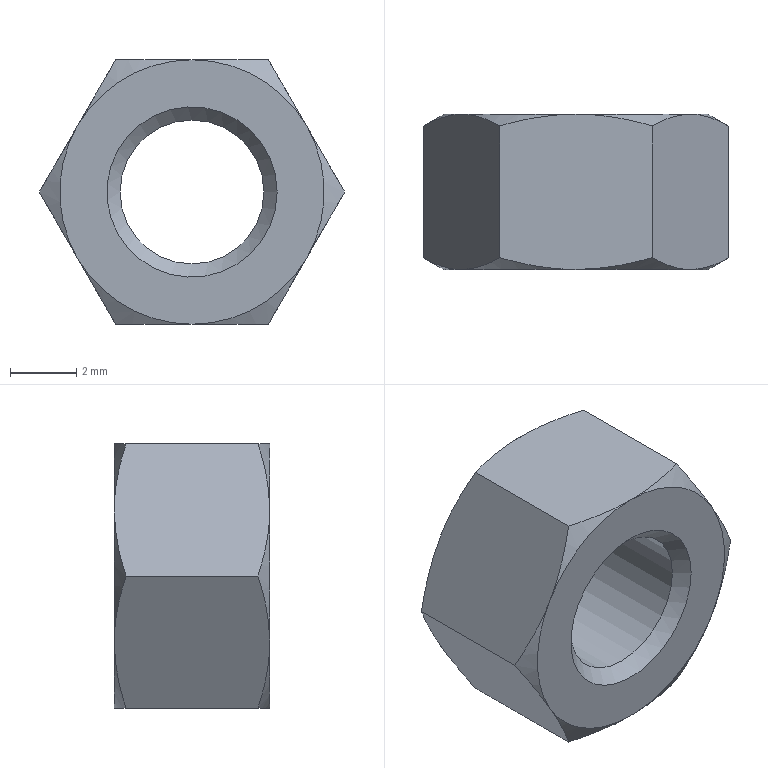Part | STEP file | solid 165 | 1 solid | 23 faces | box 9.238 x 4.7 x 8 mm | volume 187.183 mm3 | cone 14 | plane 8 | cylinder 1 | commonest cylinder face diameters 4.351 x1